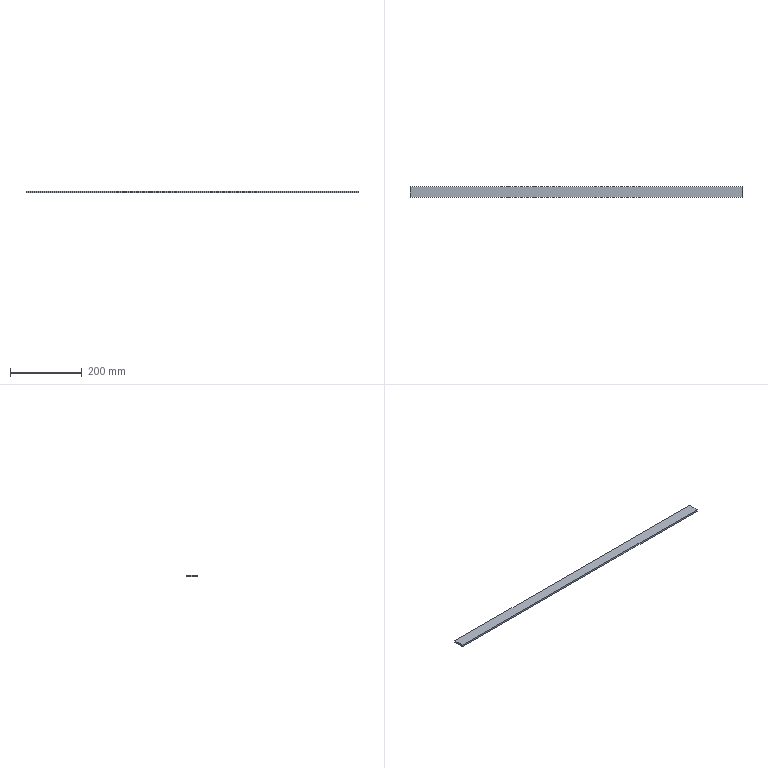Part | SolidWorks | features Extrusion 1 | 1 solid | 6 faces | box 925 x 30 x 5 mm | volume 138750 mm3 | plane 6
STEP:
#1=CARTESIAN_POINT('',(462.5,-15.,0.));
#2=VERTEX_POINT('',#1);
#3=CARTESIAN_POINT('',(462.5,15.,0.));
#4=VERTEX_POINT('',#3);
#5=CARTESIAN_POINT('',(462.5,15.,0.));
#6=DIRECTION('',(0.,1.,0.));
#7=VECTOR('',#6,1000.);
#8=LINE('',#5,#7);
#9=EDGE_CURVE('',#2,#4,#8,.T.);
#10=ORIENTED_EDGE('',*,*,#9,.T.);
#11=CARTESIAN_POINT('',(462.5,15.,5.));
#12=VERTEX_POINT('',#11);
#13=CARTESIAN_POINT('',(462.5,15.,5.));
#14=DIRECTION('',(0.,0.,-1.));
#15=VECTOR('',#14,1000.);
#16=LINE('',#13,#15);
#17=EDGE_CURVE('',#12,#4,#16,.T.);
#18=ORIENTED_EDGE('',*,*,#17,.F.);
#19=CARTESIAN_POINT('',(462.5,-15.,5.));
#20=VERTEX_POINT('',#19);
#21=CARTESIAN_POINT('',(462.5,15.,5.));
#22=DIRECTION('',(0.,1.,0.));
#23=VECTOR('',#22,1000.);
#24=LINE('',#21,#23);
#25=EDGE_CURVE('',#20,#12,#24,.T.);
#26=ORIENTED_EDGE('',*,*,#25,.F.);
#27=CARTESIAN_POINT('',(462.5,-15.,5.));
#28=DIRECTION('',(0.,0.,-1.));
#29=VECTOR('',#28,1000.);
#30=LINE('',#27,#29);
#31=EDGE_CURVE('',#20,#2,#30,.T.);
#32=ORIENTED_EDGE('',*,*,#31,.T.);
#33=EDGE_LOOP('',(#10,#18,#26,#32));
#34=FACE_OUTER_BOUND('',#33,.T.);
#35=CARTESIAN_POINT('',(462.5,15.,5.));
#36=DIRECTION('',(-1.,0.,0.));
#37=DIRECTION('',(0.,0.,1.));
#38=AXIS2_PLACEMENT_3D('',#35,#36,#37);
#39=PLANE('',#38);
#40=ADVANCED_FACE('',(#34),#39,.F.);
#41=CARTESIAN_POINT('',(-462.5,15.,0.));
#42=VERTEX_POINT('',#41);
#43=CARTESIAN_POINT('',(-462.5,15.,0.));
#44=DIRECTION('',(-1.,0.,0.));
#45=VECTOR('',#44,1000.);
#46=LINE('',#43,#45);
#47=EDGE_CURVE('',#4,#42,#46,.T.);
#48=ORIENTED_EDGE('',*,*,#47,.T.);
#49=CARTESIAN_POINT('',(-462.5,15.,5.));
#50=VERTEX_POINT('',#49);
#51=CARTESIAN_POINT('',(-462.5,15.,5.));
#52=DIRECTION('',(0.,0.,-1.));
#53=VECTOR('',#52,1000.);
#54=LINE('',#51,#53);
#55=EDGE_CURVE('',#50,#42,#54,.T.);
#56=ORIENTED_EDGE('',*,*,#55,.F.);
#57=CARTESIAN_POINT('',(-462.5,15.,5.));
#58=DIRECTION('',(-1.,0.,0.));
#59=VECTOR('',#58,1000.);
#60=LINE('',#57,#59);
#61=EDGE_CURVE('',#12,#50,#60,.T.);
#62=ORIENTED_EDGE('',*,*,#61,.F.);
#63=ORIENTED_EDGE('',*,*,#17,.T.);
#64=EDGE_LOOP('',(#48,#56,#62,#63));
#65=FACE_OUTER_BOUND('',#64,.T.);
#66=CARTESIAN_POINT('',(-462.5,15.,5.));
#67=DIRECTION('',(0.,-1.,0.));
#68=DIRECTION('',(0.,0.,-1.));
#69=AXIS2_PLACEMENT_3D('',#66,#67,#68);
#70=PLANE('',#69);
#71=ADVANCED_FACE('',(#65),#70,.F.);
#72=CARTESIAN_POINT('',(-462.5,-15.,0.));
#73=VERTEX_POINT('',#72);
#74=CARTESIAN_POINT('',(-462.5,15.,0.));
#75=DIRECTION('',(0.,-1.,0.));
#76=VECTOR('',#75,1000.);
#77=LINE('',#74,#76);
#78=EDGE_CURVE('',#42,#73,#77,.T.);
#79=ORIENTED_EDGE('',*,*,#78,.T.);
#80=CARTESIAN_POINT('',(-462.5,-15.,5.));
#81=VERTEX_POINT('',#80);
#82=CARTESIAN_POINT('',(-462.5,-15.,5.));
#83=DIRECTION('',(0.,0.,-1.));
#84=VECTOR('',#83,1000.);
#85=LINE('',#82,#84);
#86=EDGE_CURVE('',#81,#73,#85,.T.);
#87=ORIENTED_EDGE('',*,*,#86,.F.);
#88=CARTESIAN_POINT('',(-462.5,15.,5.));
#89=DIRECTION('',(0.,-1.,0.));
#90=VECTOR('',#89,1000.);
#91=LINE('',#88,#90);
#92=EDGE_CURVE('',#50,#81,#91,.T.);
#93=ORIENTED_EDGE('',*,*,#92,.F.);
#94=ORIENTED_EDGE('',*,*,#55,.T.);
#95=EDGE_LOOP('',(#79,#87,#93,#94));
#96=FACE_OUTER_BOUND('',#95,.T.);
#97=CARTESIAN_POINT('',(-462.5,15.,5.));
#98=DIRECTION('',(1.,0.,0.));
#99=DIRECTION('',(0.,0.,-1.));
#100=AXIS2_PLACEMENT_3D('',#97,#98,#99);
#101=PLANE('',#100);
#102=ADVANCED_FACE('',(#96),#101,.F.);
#103=CARTESIAN_POINT('',(-462.5,-15.,0.));
#104=DIRECTION('',(1.,0.,0.));
#105=VECTOR('',#104,1000.);
#106=LINE('',#103,#105);
#107=EDGE_CURVE('',#73,#2,#106,.T.);
#108=ORIENTED_EDGE('',*,*,#107,.T.);
#109=ORIENTED_EDGE('',*,*,#31,.F.);
#110=CARTESIAN_POINT('',(-462.5,-15.,5.));
#111=DIRECTION('',(1.,0.,0.));
#112=VECTOR('',#111,1000.);
#113=LINE('',#110,#112);
#114=EDGE_CURVE('',#81,#20,#113,.T.);
#115=ORIENTED_EDGE('',*,*,#114,.F.);
#116=ORIENTED_EDGE('',*,*,#86,.T.);
#117=EDGE_LOOP('',(#108,#109,#115,#116));
#118=FACE_OUTER_BOUND('',#117,.T.);
#119=CARTESIAN_POINT('',(-462.5,-15.,5.));
#120=DIRECTION('',(0.,1.,0.));
#121=DIRECTION('',(0.,0.,1.));
#122=AXIS2_PLACEMENT_3D('',#119,#120,#121);
#123=PLANE('',#122);
#124=ADVANCED_FACE('',(#118),#123,.F.);
#125=ORIENTED_EDGE('',*,*,#25,.T.);
#126=ORIENTED_EDGE('',*,*,#61,.T.);
#127=ORIENTED_EDGE('',*,*,#92,.T.);
#128=ORIENTED_EDGE('',*,*,#114,.T.);
#129=EDGE_LOOP('',(#125,#126,#127,#128));
#130=FACE_OUTER_BOUND('',#129,.T.);
#131=CARTESIAN_POINT('',(0.,0.,5.));
#132=DIRECTION('',(0.,0.,1.));
#133=DIRECTION('',(1.,0.,0.));
#134=AXIS2_PLACEMENT_3D('',#131,#132,#133);
#135=PLANE('',#134);
#136=ADVANCED_FACE('',(#130),#135,.T.);
#137=ORIENTED_EDGE('',*,*,#9,.F.);
#138=ORIENTED_EDGE('',*,*,#107,.F.);
#139=ORIENTED_EDGE('',*,*,#78,.F.);
#140=ORIENTED_EDGE('',*,*,#47,.F.);
#141=EDGE_LOOP('',(#137,#138,#139,#140));
#142=FACE_OUTER_BOUND('',#141,.T.);
#143=CARTESIAN_POINT('',(0.,0.,0.));
#144=DIRECTION('',(0.,0.,1.));
#145=DIRECTION('',(1.,0.,0.));
#146=AXIS2_PLACEMENT_3D('',#143,#144,#145);
#147=PLANE('',#146);
#148=ADVANCED_FACE('',(#142),#147,.F.);
#149=CLOSED_SHELL('',(#40,#71,#102,#124,#136,#148));
#150=MANIFOLD_SOLID_BREP('',#149);
#151=CARTESIAN_POINT('',(0.,0.,0.));
#152=DIRECTION('',(0.,0.,1.));
#153=DIRECTION('',(1.,0.,0.));
#154=AXIS2_PLACEMENT_3D('',#151,#152,#153);
#155=(LENGTH_UNIT()NAMED_UNIT(*)SI_UNIT(.MILLI.,.METRE.));
#156=UNCERTAINTY_MEASURE_WITH_UNIT(LENGTH_MEASURE(0.00001),#155,'','');
#157=(NAMED_UNIT(*)PLANE_ANGLE_UNIT()SI_UNIT($,.RADIAN.));
#158=(NAMED_UNIT(*)SI_UNIT($,.STERADIAN.)SOLID_ANGLE_UNIT());
#159=(GEOMETRIC_REPRESENTATION_CONTEXT(3)GLOBAL_UNCERTAINTY_ASSIGNED_CONTEXT((#156))GLOBAL_UNIT_ASSIGNED_CONTEXT((#155,#157,#158))REPRESENTATION_CONTEXT('',''));
#160=ADVANCED_BREP_SHAPE_REPRESENTATION('',(#150,#154),#159);